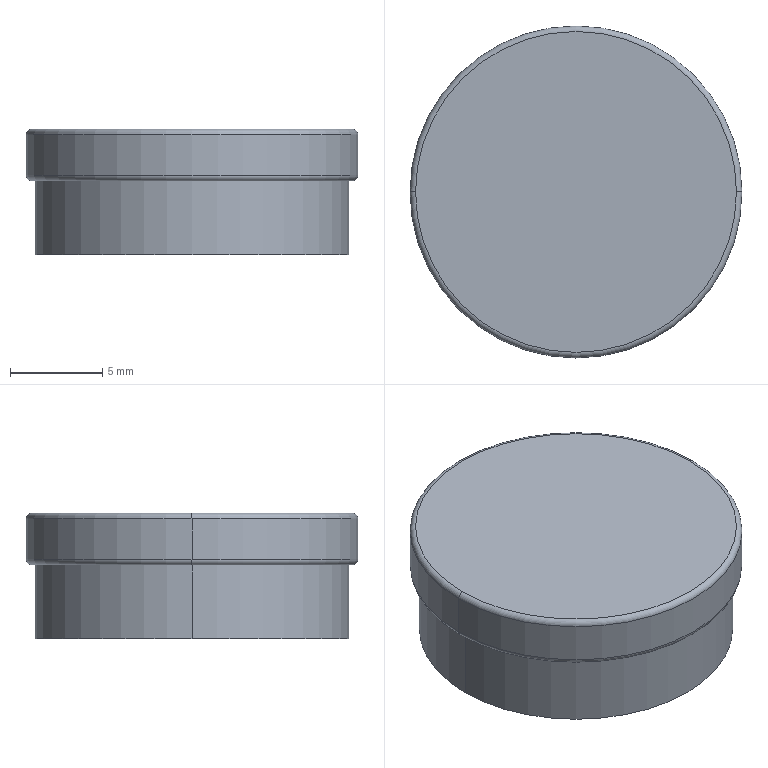Part | SolidWorks | features Cut 1, Extrusion 1, Fillet 1, ICE 1 | 1 solid | 14 faces | box 18 x 18 x 6.8 mm | volume 1583 mm3 | cylinder 6 | torus 4 | plane 4 | commonest cylinder face diameters 3 x2 17 x2 18 x2
STEP:
#1=CARTESIAN_POINT('',(1.5,0.,5.));
#2=VERTEX_POINT('',#1);
#3=CARTESIAN_POINT('',(-1.5,0.,5.));
#4=VERTEX_POINT('',#3);
#5=CARTESIAN_POINT('',(0.,0.,5.));
#6=DIRECTION('',(0.,0.,-1.));
#7=DIRECTION('',(-1.,0.,0.));
#8=AXIS2_PLACEMENT_3D('',#5,#6,#7);
#9=CIRCLE('',#8,1.5);
#10=EDGE_CURVE('',#2,#4,#9,.T.);
#11=ORIENTED_EDGE('',*,*,#10,.F.);
#12=CARTESIAN_POINT('',(1.5,0.,0.));
#13=VERTEX_POINT('',#12);
#14=CARTESIAN_POINT('',(1.5,0.,5.));
#15=DIRECTION('',(0.,0.,-1.));
#16=VECTOR('',#15,1000.);
#17=LINE('',#14,#16);
#18=EDGE_CURVE('',#2,#13,#17,.T.);
#19=ORIENTED_EDGE('',*,*,#18,.T.);
#20=CARTESIAN_POINT('',(-1.5,0.,0.));
#21=VERTEX_POINT('',#20);
#22=CARTESIAN_POINT('',(0.,0.,0.));
#23=DIRECTION('',(0.,0.,-1.));
#24=DIRECTION('',(-1.,0.,0.));
#25=AXIS2_PLACEMENT_3D('',#22,#23,#24);
#26=CIRCLE('',#25,1.5);
#27=EDGE_CURVE('',#13,#21,#26,.T.);
#28=ORIENTED_EDGE('',*,*,#27,.T.);
#29=CARTESIAN_POINT('',(-1.5,0.,5.));
#30=DIRECTION('',(0.,0.,-1.));
#31=VECTOR('',#30,1000.);
#32=LINE('',#29,#31);
#33=EDGE_CURVE('',#4,#21,#32,.T.);
#34=ORIENTED_EDGE('',*,*,#33,.F.);
#35=EDGE_LOOP('',(#11,#19,#28,#34));
#36=FACE_OUTER_BOUND('',#35,.T.);
#37=CARTESIAN_POINT('',(0.,0.,5.));
#38=DIRECTION('',(0.,0.,-1.));
#39=DIRECTION('',(-1.,0.,0.));
#40=AXIS2_PLACEMENT_3D('',#37,#38,#39);
#41=CYLINDRICAL_SURFACE('',#40,1.5);
#42=ADVANCED_FACE('',(#36),#41,.F.);
#43=CARTESIAN_POINT('',(-9.,0.,6.5));
#44=VERTEX_POINT('',#43);
#45=CARTESIAN_POINT('',(9.,0.,6.5));
#46=VERTEX_POINT('',#45);
#47=CARTESIAN_POINT('',(0.,0.,6.5));
#48=DIRECTION('',(0.,0.,-1.));
#49=DIRECTION('',(1.,0.,0.));
#50=AXIS2_PLACEMENT_3D('',#47,#48,#49);
#51=CIRCLE('',#50,9.);
#52=EDGE_CURVE('',#44,#46,#51,.T.);
#53=ORIENTED_EDGE('',*,*,#52,.F.);
#54=CARTESIAN_POINT('',(-8.7,0.,6.8));
#55=VERTEX_POINT('',#54);
#56=CARTESIAN_POINT('',(-8.7,0.,6.5));
#57=DIRECTION('',(0.,1.,0.));
#58=DIRECTION('',(-1.,0.,0.));
#59=AXIS2_PLACEMENT_3D('',#56,#57,#58);
#60=CIRCLE('',#59,0.3);
#61=EDGE_CURVE('',#44,#55,#60,.T.);
#62=ORIENTED_EDGE('',*,*,#61,.T.);
#63=CARTESIAN_POINT('',(8.7,0.,6.8));
#64=VERTEX_POINT('',#63);
#65=CARTESIAN_POINT('',(0.,0.,6.8));
#66=DIRECTION('',(0.,0.,1.));
#67=DIRECTION('',(1.,0.,0.));
#68=AXIS2_PLACEMENT_3D('',#65,#66,#67);
#69=CIRCLE('',#68,8.7);
#70=EDGE_CURVE('',#64,#55,#69,.T.);
#71=ORIENTED_EDGE('',*,*,#70,.F.);
#72=CARTESIAN_POINT('',(8.7,0.,6.5));
#73=DIRECTION('',(0.,-1.,0.));
#74=DIRECTION('',(0.,0.,-1.));
#75=AXIS2_PLACEMENT_3D('',#72,#73,#74);
#76=CIRCLE('',#75,0.3);
#77=EDGE_CURVE('',#46,#64,#76,.T.);
#78=ORIENTED_EDGE('',*,*,#77,.F.);
#79=EDGE_LOOP('',(#53,#62,#71,#78));
#80=FACE_OUTER_BOUND('',#79,.T.);
#81=CARTESIAN_POINT('',(0.,0.,6.5));
#82=DIRECTION('',(0.,0.,1.));
#83=DIRECTION('',(1.,0.,0.));
#84=AXIS2_PLACEMENT_3D('',#81,#82,#83);
#85=TOROIDAL_SURFACE('',#84,8.7,0.3);
#86=ADVANCED_FACE('',(#80),#85,.T.);
#87=CARTESIAN_POINT('',(-8.7,0.,4.));
#88=VERTEX_POINT('',#87);
#89=CARTESIAN_POINT('',(8.7,0.,4.));
#90=VERTEX_POINT('',#89);
#91=CARTESIAN_POINT('',(0.,0.,4.));
#92=DIRECTION('',(0.,0.,-1.));
#93=DIRECTION('',(1.,0.,0.));
#94=AXIS2_PLACEMENT_3D('',#91,#92,#93);
#95=CIRCLE('',#94,8.7);
#96=EDGE_CURVE('',#88,#90,#95,.T.);
#97=ORIENTED_EDGE('',*,*,#96,.F.);
#98=CARTESIAN_POINT('',(-9.,0.,4.3));
#99=VERTEX_POINT('',#98);
#100=CARTESIAN_POINT('',(-8.7,0.,4.3));
#101=DIRECTION('',(0.,1.,0.));
#102=DIRECTION('',(-1.,0.,0.));
#103=AXIS2_PLACEMENT_3D('',#100,#101,#102);
#104=CIRCLE('',#103,0.3);
#105=EDGE_CURVE('',#88,#99,#104,.T.);
#106=ORIENTED_EDGE('',*,*,#105,.T.);
#107=CARTESIAN_POINT('',(9.,0.,4.3));
#108=VERTEX_POINT('',#107);
#109=CARTESIAN_POINT('',(0.,0.,4.3));
#110=DIRECTION('',(0.,0.,1.));
#111=DIRECTION('',(1.,0.,0.));
#112=AXIS2_PLACEMENT_3D('',#109,#110,#111);
#113=CIRCLE('',#112,9.);
#114=EDGE_CURVE('',#108,#99,#113,.T.);
#115=ORIENTED_EDGE('',*,*,#114,.F.);
#116=CARTESIAN_POINT('',(8.7,0.,4.3));
#117=DIRECTION('',(0.,-1.,0.));
#118=DIRECTION('',(0.,0.,-1.));
#119=AXIS2_PLACEMENT_3D('',#116,#117,#118);
#120=CIRCLE('',#119,0.3);
#121=EDGE_CURVE('',#90,#108,#120,.T.);
#122=ORIENTED_EDGE('',*,*,#121,.F.);
#123=EDGE_LOOP('',(#97,#106,#115,#122));
#124=FACE_OUTER_BOUND('',#123,.T.);
#125=CARTESIAN_POINT('',(0.,0.,4.3));
#126=DIRECTION('',(0.,0.,1.));
#127=DIRECTION('',(1.,0.,0.));
#128=AXIS2_PLACEMENT_3D('',#125,#126,#127);
#129=TOROIDAL_SURFACE('',#128,8.7,0.3);
#130=ADVANCED_FACE('',(#124),#129,.T.);
#131=ORIENTED_EDGE('',*,*,#52,.T.);
#132=CARTESIAN_POINT('',(9.,0.,6.8));
#133=DIRECTION('',(0.,0.,-1.));
#134=VECTOR('',#133,1000.);
#135=LINE('',#132,#134);
#136=EDGE_CURVE('',#46,#108,#135,.T.);
#137=ORIENTED_EDGE('',*,*,#136,.T.);
#138=ORIENTED_EDGE('',*,*,#114,.T.);
#139=CARTESIAN_POINT('',(-9.,0.,6.8));
#140=DIRECTION('',(0.,0.,-1.));
#141=VECTOR('',#140,1000.);
#142=LINE('',#139,#141);
#143=EDGE_CURVE('',#44,#99,#142,.T.);
#144=ORIENTED_EDGE('',*,*,#143,.F.);
#145=EDGE_LOOP('',(#131,#137,#138,#144));
#146=FACE_OUTER_BOUND('',#145,.T.);
#147=CARTESIAN_POINT('',(0.,0.,6.8));
#148=DIRECTION('',(0.,0.,-1.));
#149=DIRECTION('',(-1.,0.,0.));
#150=AXIS2_PLACEMENT_3D('',#147,#148,#149);
#151=CYLINDRICAL_SURFACE('',#150,9.);
#152=ADVANCED_FACE('',(#146),#151,.T.);
#153=CARTESIAN_POINT('',(8.5,0.,4.));
#154=VERTEX_POINT('',#153);
#155=CARTESIAN_POINT('',(-8.5,0.,4.));
#156=VERTEX_POINT('',#155);
#157=CARTESIAN_POINT('',(0.,0.,4.));
#158=DIRECTION('',(0.,0.,1.));
#159=DIRECTION('',(1.,0.,0.));
#160=AXIS2_PLACEMENT_3D('',#157,#158,#159);
#161=CIRCLE('',#160,8.5);
#162=EDGE_CURVE('',#154,#156,#161,.T.);
#163=ORIENTED_EDGE('',*,*,#162,.F.);
#164=CARTESIAN_POINT('',(8.5,0.,0.));
#165=VERTEX_POINT('',#164);
#166=CARTESIAN_POINT('',(8.5,0.,4.));
#167=DIRECTION('',(0.,0.,-1.));
#168=VECTOR('',#167,1000.);
#169=LINE('',#166,#168);
#170=EDGE_CURVE('',#154,#165,#169,.T.);
#171=ORIENTED_EDGE('',*,*,#170,.T.);
#172=CARTESIAN_POINT('',(-8.5,0.,0.));
#173=VERTEX_POINT('',#172);
#174=CARTESIAN_POINT('',(0.,0.,0.));
#175=DIRECTION('',(0.,0.,1.));
#176=DIRECTION('',(1.,0.,0.));
#177=AXIS2_PLACEMENT_3D('',#174,#175,#176);
#178=CIRCLE('',#177,8.5);
#179=EDGE_CURVE('',#165,#173,#178,.T.);
#180=ORIENTED_EDGE('',*,*,#179,.T.);
#181=CARTESIAN_POINT('',(-8.5,0.,4.));
#182=DIRECTION('',(0.,0.,-1.));
#183=VECTOR('',#182,1000.);
#184=LINE('',#181,#183);
#185=EDGE_CURVE('',#156,#173,#184,.T.);
#186=ORIENTED_EDGE('',*,*,#185,.F.);
#187=EDGE_LOOP('',(#163,#171,#180,#186));
#188=FACE_OUTER_BOUND('',#187,.T.);
#189=CARTESIAN_POINT('',(0.,0.,4.));
#190=DIRECTION('',(0.,0.,-1.));
#191=DIRECTION('',(-1.,0.,0.));
#192=AXIS2_PLACEMENT_3D('',#189,#190,#191);
#193=CYLINDRICAL_SURFACE('',#192,8.5);
#194=ADVANCED_FACE('',(#188),#193,.T.);
#195=ORIENTED_EDGE('',*,*,#170,.F.);
#196=CARTESIAN_POINT('',(0.,0.,4.));
#197=DIRECTION('',(0.,0.,1.));
#198=DIRECTION('',(1.,0.,0.));
#199=AXIS2_PLACEMENT_3D('',#196,#197,#198);
#200=CIRCLE('',#199,8.5);
#201=EDGE_CURVE('',#156,#154,#200,.T.);
#202=ORIENTED_EDGE('',*,*,#201,.F.);
#203=ORIENTED_EDGE('',*,*,#185,.T.);
#204=CARTESIAN_POINT('',(0.,0.,0.));
#205=DIRECTION('',(0.,0.,1.));
#206=DIRECTION('',(1.,0.,0.));
#207=AXIS2_PLACEMENT_3D('',#204,#205,#206);
#208=CIRCLE('',#207,8.5);
#209=EDGE_CURVE('',#173,#165,#208,.T.);
#210=ORIENTED_EDGE('',*,*,#209,.T.);
#211=EDGE_LOOP('',(#195,#202,#203,#210));
#212=FACE_OUTER_BOUND('',#211,.T.);
#213=CARTESIAN_POINT('',(0.,0.,4.));
#214=DIRECTION('',(0.,0.,-1.));
#215=DIRECTION('',(-1.,0.,0.));
#216=AXIS2_PLACEMENT_3D('',#213,#214,#215);
#217=CYLINDRICAL_SURFACE('',#216,8.5);
#218=ADVANCED_FACE('',(#212),#217,.T.);
#219=CARTESIAN_POINT('',(0.,0.,0.));
#220=DIRECTION('',(0.,0.,-1.));
#221=DIRECTION('',(-1.,0.,0.));
#222=AXIS2_PLACEMENT_3D('',#219,#220,#221);
#223=CIRCLE('',#222,1.5);
#224=EDGE_CURVE('',#21,#13,#223,.T.);
#225=ORIENTED_EDGE('',*,*,#224,.F.);
#226=ORIENTED_EDGE('',*,*,#27,.F.);
#227=EDGE_LOOP('',(#225,#226));
#228=FACE_BOUND('',#227,.T.);
#229=ORIENTED_EDGE('',*,*,#209,.F.);
#230=ORIENTED_EDGE('',*,*,#179,.F.);
#231=EDGE_LOOP('',(#229,#230));
#232=FACE_OUTER_BOUND('',#231,.T.);
#233=CARTESIAN_POINT('',(0.,0.,0.));
#234=DIRECTION('',(0.,0.,1.));
#235=DIRECTION('',(1.,0.,0.));
#236=AXIS2_PLACEMENT_3D('',#233,#234,#235);
#237=PLANE('',#236);
#238=ADVANCED_FACE('',(#228,#232),#237,.F.);
#239=ORIENTED_EDGE('',*,*,#136,.F.);
#240=CARTESIAN_POINT('',(0.,0.,6.5));
#241=DIRECTION('',(0.,0.,-1.));
#242=DIRECTION('',(1.,0.,0.));
#243=AXIS2_PLACEMENT_3D('',#240,#241,#242);
#244=CIRCLE('',#243,9.);
#245=EDGE_CURVE('',#46,#44,#244,.T.);
#246=ORIENTED_EDGE('',*,*,#245,.T.);
#247=ORIENTED_EDGE('',*,*,#143,.T.);
#248=CARTESIAN_POINT('',(0.,0.,4.3));
#249=DIRECTION('',(0.,0.,1.));
#250=DIRECTION('',(1.,0.,0.));
#251=AXIS2_PLACEMENT_3D('',#248,#249,#250);
#252=CIRCLE('',#251,9.);
#253=EDGE_CURVE('',#99,#108,#252,.T.);
#254=ORIENTED_EDGE('',*,*,#253,.T.);
#255=EDGE_LOOP('',(#239,#246,#247,#254));
#256=FACE_OUTER_BOUND('',#255,.T.);
#257=CARTESIAN_POINT('',(0.,0.,6.8));
#258=DIRECTION('',(0.,0.,-1.));
#259=DIRECTION('',(-1.,0.,0.));
#260=AXIS2_PLACEMENT_3D('',#257,#258,#259);
#261=CYLINDRICAL_SURFACE('',#260,9.);
#262=ADVANCED_FACE('',(#256),#261,.T.);
#263=ORIENTED_EDGE('',*,*,#70,.T.);
#264=CARTESIAN_POINT('',(0.,0.,6.8));
#265=DIRECTION('',(0.,0.,1.));
#266=DIRECTION('',(1.,0.,0.));
#267=AXIS2_PLACEMENT_3D('',#264,#265,#266);
#268=CIRCLE('',#267,8.7);
#269=EDGE_CURVE('',#55,#64,#268,.T.);
#270=ORIENTED_EDGE('',*,*,#269,.T.);
#271=EDGE_LOOP('',(#263,#270));
#272=FACE_OUTER_BOUND('',#271,.T.);
#273=CARTESIAN_POINT('',(0.,0.,6.8));
#274=DIRECTION('',(0.,0.,1.));
#275=DIRECTION('',(1.,0.,0.));
#276=AXIS2_PLACEMENT_3D('',#273,#274,#275);
#277=PLANE('',#276);
#278=ADVANCED_FACE('',(#272),#277,.T.);
#279=CARTESIAN_POINT('',(0.,0.,4.));
#280=DIRECTION('',(0.,0.,-1.));
#281=DIRECTION('',(1.,0.,0.));
#282=AXIS2_PLACEMENT_3D('',#279,#280,#281);
#283=CIRCLE('',#282,8.7);
#284=EDGE_CURVE('',#90,#88,#283,.T.);
#285=ORIENTED_EDGE('',*,*,#284,.T.);
#286=ORIENTED_EDGE('',*,*,#96,.T.);
#287=EDGE_LOOP('',(#285,#286));
#288=FACE_OUTER_BOUND('',#287,.T.);
#289=ORIENTED_EDGE('',*,*,#201,.T.);
#290=ORIENTED_EDGE('',*,*,#162,.T.);
#291=EDGE_LOOP('',(#289,#290));
#292=FACE_BOUND('',#291,.T.);
#293=CARTESIAN_POINT('',(0.,0.,4.));
#294=DIRECTION('',(0.,0.,1.));
#295=DIRECTION('',(1.,0.,0.));
#296=AXIS2_PLACEMENT_3D('',#293,#294,#295);
#297=PLANE('',#296);
#298=ADVANCED_FACE('',(#288,#292),#297,.F.);
#299=ORIENTED_EDGE('',*,*,#105,.F.);
#300=ORIENTED_EDGE('',*,*,#284,.F.);
#301=ORIENTED_EDGE('',*,*,#121,.T.);
#302=ORIENTED_EDGE('',*,*,#253,.F.);
#303=EDGE_LOOP('',(#299,#300,#301,#302));
#304=FACE_OUTER_BOUND('',#303,.T.);
#305=CARTESIAN_POINT('',(0.,0.,4.3));
#306=DIRECTION('',(0.,0.,1.));
#307=DIRECTION('',(1.,0.,0.));
#308=AXIS2_PLACEMENT_3D('',#305,#306,#307);
#309=TOROIDAL_SURFACE('',#308,8.7,0.3);
#310=ADVANCED_FACE('',(#304),#309,.T.);
#311=ORIENTED_EDGE('',*,*,#61,.F.);
#312=ORIENTED_EDGE('',*,*,#245,.F.);
#313=ORIENTED_EDGE('',*,*,#77,.T.);
#314=ORIENTED_EDGE('',*,*,#269,.F.);
#315=EDGE_LOOP('',(#311,#312,#313,#314));
#316=FACE_OUTER_BOUND('',#315,.T.);
#317=CARTESIAN_POINT('',(0.,0.,6.5));
#318=DIRECTION('',(0.,0.,1.));
#319=DIRECTION('',(1.,0.,0.));
#320=AXIS2_PLACEMENT_3D('',#317,#318,#319);
#321=TOROIDAL_SURFACE('',#320,8.7,0.3);
#322=ADVANCED_FACE('',(#316),#321,.T.);
#323=ORIENTED_EDGE('',*,*,#18,.F.);
#324=CARTESIAN_POINT('',(0.,0.,5.));
#325=DIRECTION('',(0.,0.,-1.));
#326=DIRECTION('',(-1.,0.,0.));
#327=AXIS2_PLACEMENT_3D('',#324,#325,#326);
#328=CIRCLE('',#327,1.5);
#329=EDGE_CURVE('',#4,#2,#328,.T.);
#330=ORIENTED_EDGE('',*,*,#329,.F.);
#331=ORIENTED_EDGE('',*,*,#33,.T.);
#332=ORIENTED_EDGE('',*,*,#224,.T.);
#333=EDGE_LOOP('',(#323,#330,#331,#332));
#334=FACE_OUTER_BOUND('',#333,.T.);
#335=CARTESIAN_POINT('',(0.,0.,5.));
#336=DIRECTION('',(0.,0.,-1.));
#337=DIRECTION('',(-1.,0.,0.));
#338=AXIS2_PLACEMENT_3D('',#335,#336,#337);
#339=CYLINDRICAL_SURFACE('',#338,1.5);
#340=ADVANCED_FACE('',(#334),#339,.F.);
#341=ORIENTED_EDGE('',*,*,#329,.T.);
#342=ORIENTED_EDGE('',*,*,#10,.T.);
#343=EDGE_LOOP('',(#341,#342));
#344=FACE_OUTER_BOUND('',#343,.T.);
#345=CARTESIAN_POINT('',(0.,0.,5.));
#346=DIRECTION('',(0.,0.,-1.));
#347=DIRECTION('',(-1.,0.,0.));
#348=AXIS2_PLACEMENT_3D('',#345,#346,#347);
#349=PLANE('',#348);
#350=ADVANCED_FACE('',(#344),#349,.T.);
#351=CLOSED_SHELL('',(#42,#86,#130,#152,#194,#218,#238,#262,#278,#298,#310,#322,#340,#350));
#352=MANIFOLD_SOLID_BREP('',#351);
#353=CARTESIAN_POINT('',(0.,0.,0.));
#354=DIRECTION('',(0.,0.,1.));
#355=DIRECTION('',(1.,0.,0.));
#356=AXIS2_PLACEMENT_3D('',#353,#354,#355);
#357=(LENGTH_UNIT()NAMED_UNIT(*)SI_UNIT(.MILLI.,.METRE.));
#358=UNCERTAINTY_MEASURE_WITH_UNIT(LENGTH_MEASURE(0.00001),#357,'','');
#359=(NAMED_UNIT(*)PLANE_ANGLE_UNIT()SI_UNIT($,.RADIAN.));
#360=(NAMED_UNIT(*)SI_UNIT($,.STERADIAN.)SOLID_ANGLE_UNIT());
#361=(GEOMETRIC_REPRESENTATION_CONTEXT(3)GLOBAL_UNCERTAINTY_ASSIGNED_CONTEXT((#358))GLOBAL_UNIT_ASSIGNED_CONTEXT((#357,#359,#360))REPRESENTATION_CONTEXT('',''));
#362=ADVANCED_BREP_SHAPE_REPRESENTATION('',(#352,#356),#361);